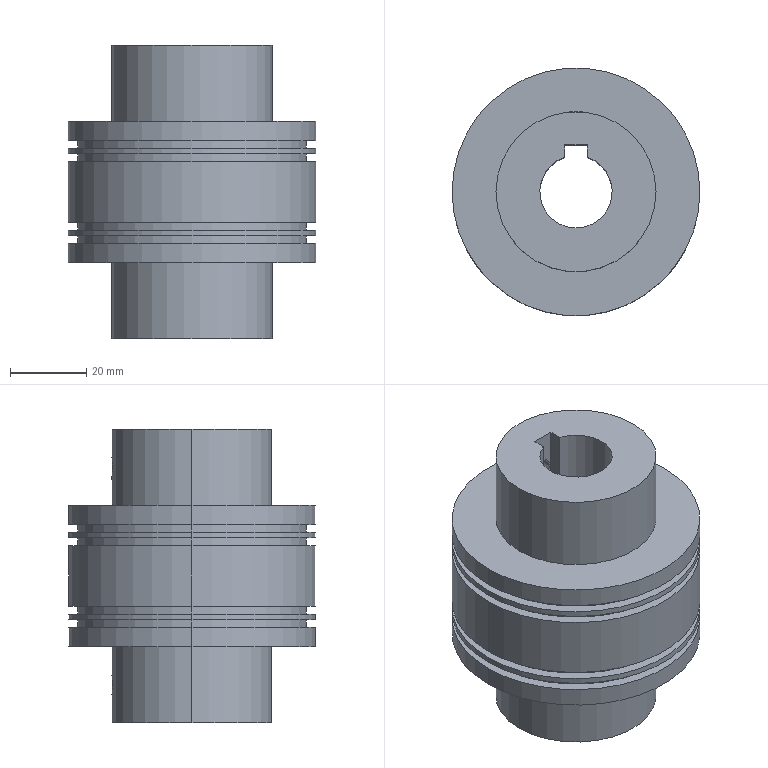Part | STEP file | Coupling CPSWWKΦ19-Φ19 (high-rigidity diaphragm type) | 1 solid | 43 faces | box 65 x 65 x 77 mm | volume 150728 mm3 | cylinder 28 | plane 15 | commonest cylinder face diameters 65 x10 60 x8 5 x4 42 x4 19 x2